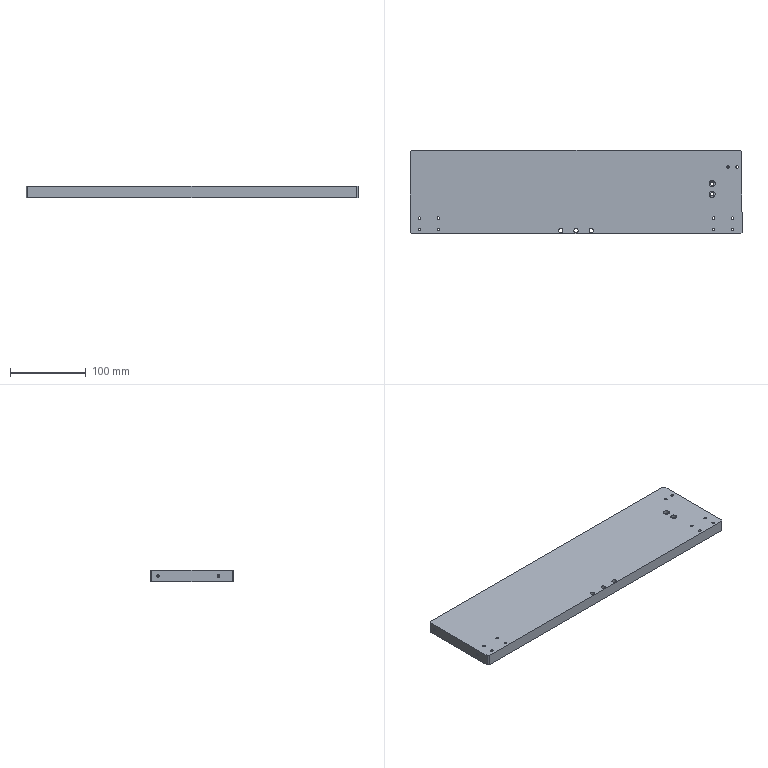Part | STEP file | FBDS-CS-030 | 1 solid | 88 faces | box 438 x 110 x 15 mm | volume 713481 mm3 | cylinder 52 | cone 20 | plane 16 | commonest cylinder face diameters 3.3 x32 5.5 x6 2.5 x4 4.5 x4 8 x4 4 x2